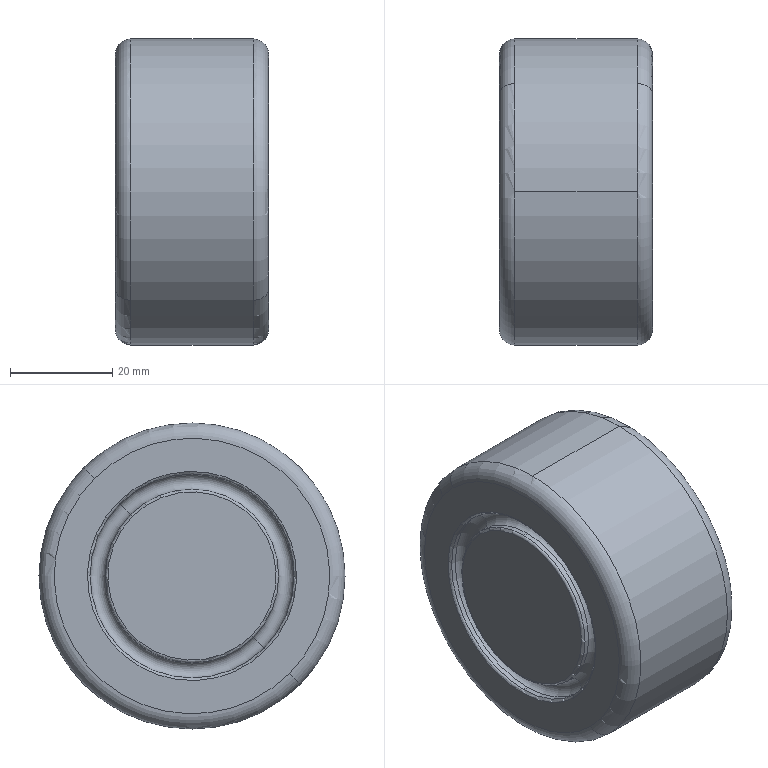Part | STEP file | ASND-0110-E63-HLTP01Clogo.sldasm-Part-214 | 1 solid | 30 faces | box 30 x 60 x 60 mm | volume 82218 mm3 | torus 16 | cylinder 10 | plane 4 | commonest cylinder face diameters 34 x4 40 x4 60 x2